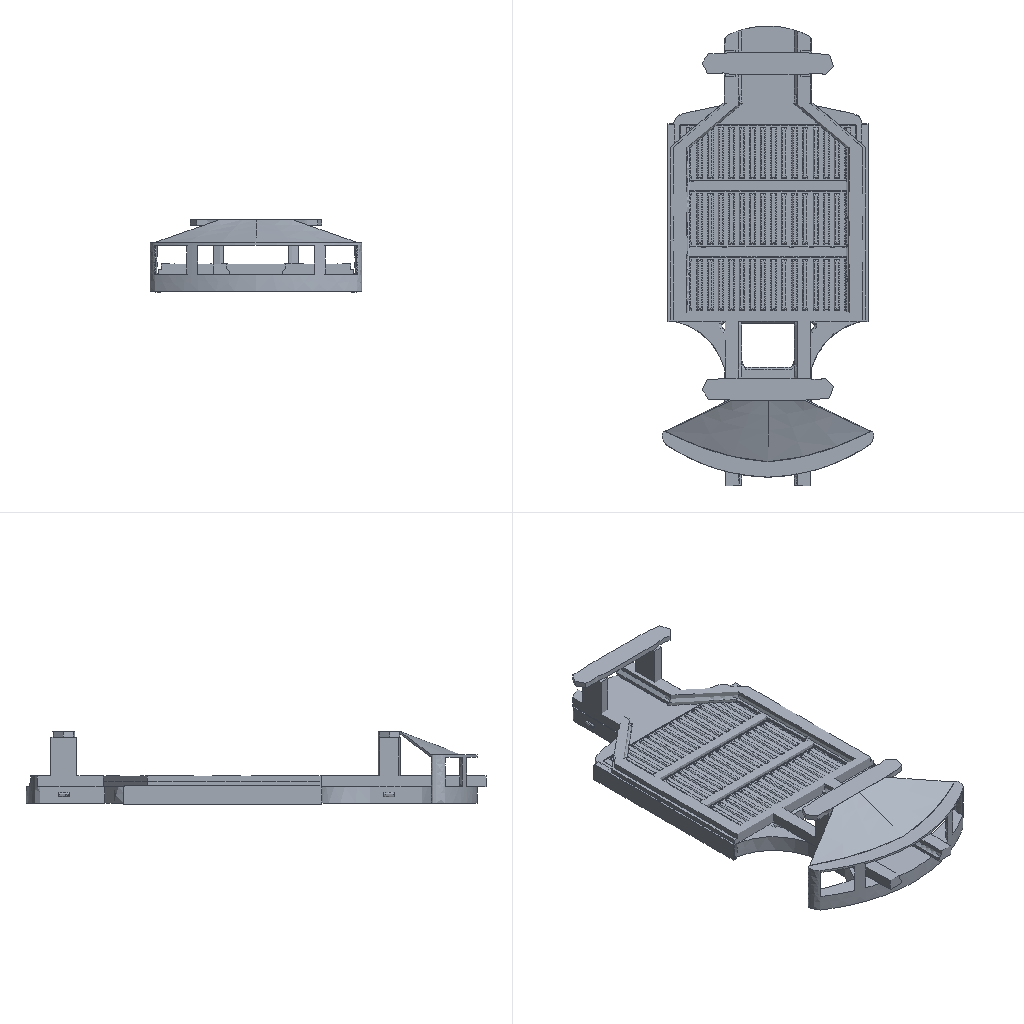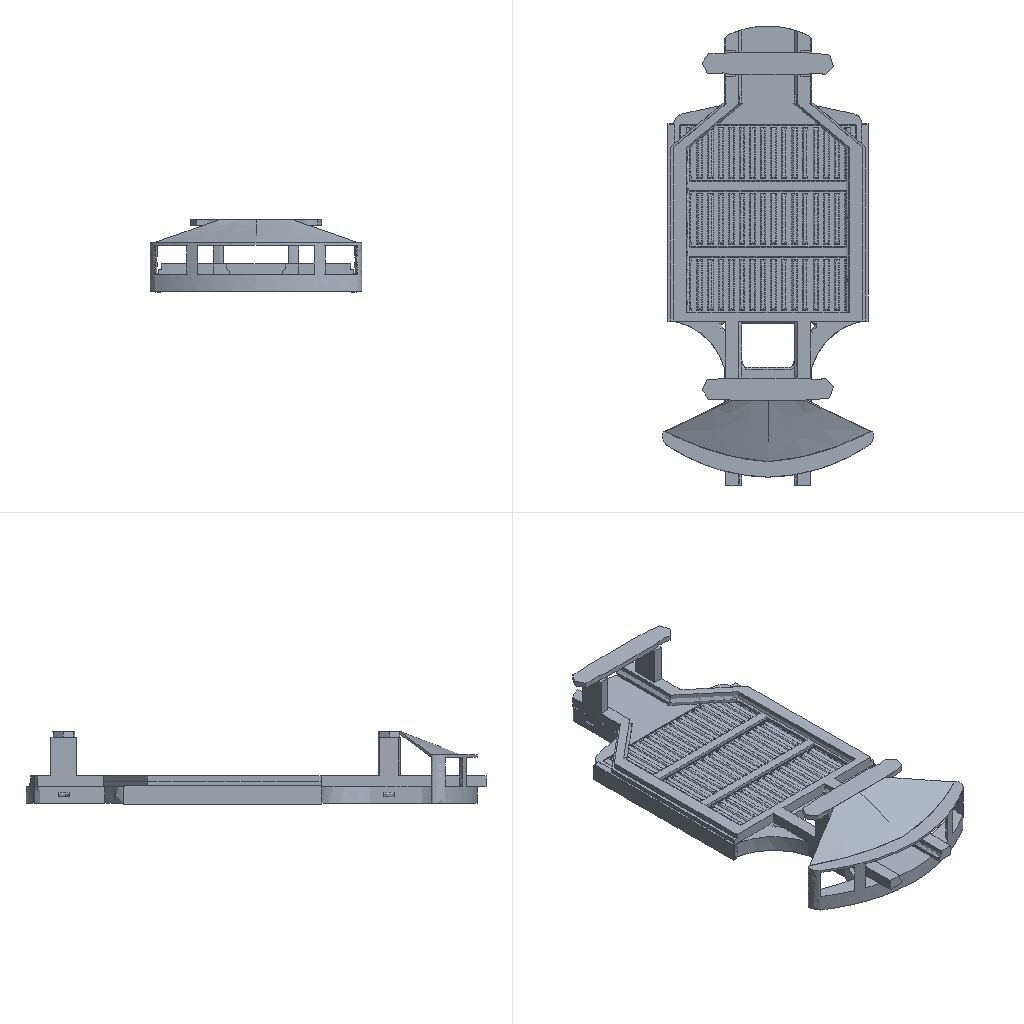Simulation study | ansys workbench
Set-up summary:
category,name,step,type,value,unit,region
solver,ansys_mapdl
solver,version,,,22.1
solver,version,,,22.1
solver,version,,,22.1
solver,version,,,22.1
units,MPA,,stated
analysis,deck1,,static,static
load_step,requested,,,1
analysis,nlgeom,,,False
mesh,nodes,,,275266
mesh,elements,,,186698
element_type,ANSYS 187 (type 1),,solid,173485
element_type,ANSYS 186 (type 2),,solid,9
element_type,ANSYS 186 (type 3),,solid,9
element_type,ANSYS 174 (type 4),,contact,6
element_type,ANSYS 170 (type 5),,target,6
element_type,ANSYS 154 (type 6),,surface,13183
load,load commands in deck,,count,3
bc,support commands in deck,,count,1
named_set,_FIXEDSU,,component
analysis,deck2,,static,static
load_step,requested,,,1
analysis,nlgeom,,,False
mesh,nodes,,,275266
mesh,elements,,,173804
element_type,ANSYS 187 (type 1),,solid,173485
element_type,ANSYS 186 (type 2),,solid,9
element_type,ANSYS 186 (type 3),,solid,9
element_type,ANSYS 174 (type 4),,contact,6
element_type,ANSYS 170 (type 5),,target,6
element_type,ANSYS 154 (type 6),,surface,289
load,load commands in deck,,count,3
bc,support commands in deck,,count,1
named_set,_FIXEDSU,,component
analysis,deck3,,static,static
load_step,requested,,,1
analysis,nlgeom,,,False
mesh,nodes,,,275267
mesh,elements,,,191421
element_type,ANSYS 187 (type 1),,solid,173485
element_type,ANSYS 186 (type 2),,solid,9
element_type,ANSYS 186 (type 3),,solid,9
element_type,ANSYS 174 (type 4),,contact,6
element_type,ANSYS 170 (type 5),,target,6
element_type,ANSYS 174 (type 6),,contact,4583
element_type,ANSYS 170 (type 7),,target,0
element_type,ANSYS 154 (type 8),,surface,434
element_type,ANSYS 154 (type 9),,surface,12889
load,load commands in deck,,count,9
bc,support commands in deck,,count,1
named_set,_FIXEDSU,,component
analysis,deck4,,static,static
load_step,requested,,,1
analysis,nlgeom,,,False
mesh,nodes,,,274989
mesh,elements,,,186819
element_type,ANSYS 187 (type 1),,solid,173220
element_type,ANSYS 186 (type 2),,solid,12
element_type,ANSYS 186 (type 3),,solid,12
element_type,ANSYS 174 (type 4),,contact,8
element_type,ANSYS 170 (type 5),,target,8
element_type,ANSYS 174 (type 6),,contact,13559
element_type,ANSYS 170 (type 7),,target,0
load,load commands in deck,,count,3
bc,support commands in deck,,count,1
named_set,_FIXEDSU,,component
material,1,,in results
material,2,,in results
material,3,,in results
material,1,,in results
material,2,,in results
material,3,,in results
material,1,,in results
material,2,,in results
material,3,,in results
material,1,,in results
material,2,,in results
material,3,,in results
check,setup vs results,,match,13183 surface effect element(s) are not in the reader's mesh and were not compared
check,setup vs results,,match,289 surface effect element(s) are not in the reader's mesh and were not compared
check,setup vs results,,match,results also hold 0 node(s) and 1 element(s) the deck makes with ['EN']; those were not compared; 1 node(s) the solver created internally for pilot nodes (solve.out) are in the results only; 13323 surface effect element(s) are not in the reader's mesh and were not compared
check,setup vs results,,match,results also hold 0 node(s) and 1 element(s) the deck makes with ['EN']; those were not compared; 1 node(s) the solver created internally for pilot nodes (solve.out) are in the results only
Results summary:
result,analysis,,,static
result,last_loadstep,,,1
result,primary field,,,displacement
result,reaction total,1,FX,4e-06,N
result,reaction total,1,FY,-9e-06,N
result,reaction total,1,FZ,500000,N
result,mass,,,7.727,"NMM: mm, ton, N, s, mV, mA, degC"
result,analysis,,,static
result,last_loadstep,,,1
result,primary field,,,displacement
result,reaction total,1,FX,0.0,N
result,reaction total,1,FY,-5000000,N
result,reaction total,1,FZ,1e-06,N
result,mass,,,7.727,"NMM: mm, ton, N, s, mV, mA, degC"
result,analysis,,,static
result,last_loadstep,,,1
result,primary field,,,displacement
result,reaction total,1,FX,2e-06,N
result,reaction total,1,FY,-499999.999,N
result,reaction total,1,FZ,500000,N
result,mass,,,7.727,"NMM: mm, ton, N, s, mV, mA, degC"
result,analysis,,,static
result,last_loadstep,,,1
result,primary field,,,displacement
result,reaction total,1,FX,-0.00015,N
result,reaction total,1,FY,-0.000214,N
result,reaction total,1,FZ,2.8e-05,N
result,mass,,,7.727,"NMM: mm, ton, N, s, mV, mA, degC"